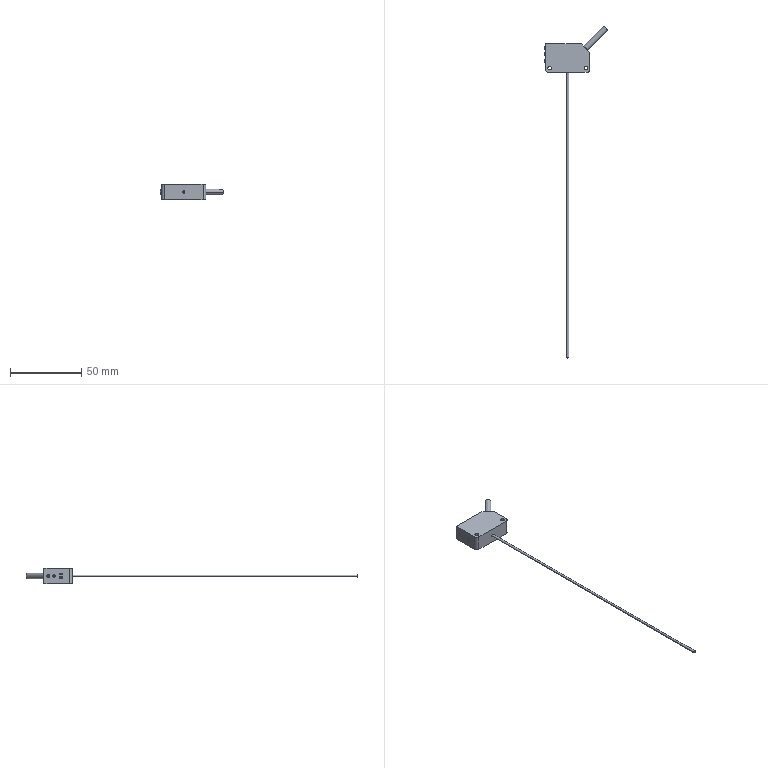Part | SolidWorks | features BaseBody 1 | 1 solid | 39 faces | box 44.556 x 232.556 x 10.8 mm | volume 6994 mm3 | cylinder 18 | plane 14 | spline 7 | commonest cylinder face diameters 2 x6 2.5 x4 4 x4 1 x2 1.5 x2
STEP:
#1=CARTESIAN_POINT('',(-0.6496,0.3346,0.03937));
#2=VERTEX_POINT('',#1);
#3=CARTESIAN_POINT('',(-0.6496,0.315,0.05906));
#4=VERTEX_POINT('',#3);
#5=CARTESIAN_POINT('',(-0.6496,0.3346,0.03937));
#6=CARTESIAN_POINT('',(-0.6496,0.3346,0.0509));
#7=CARTESIAN_POINT('',(-0.6496,0.3265,0.05906));
#8=CARTESIAN_POINT('',(-0.6496,0.315,0.05906));
#9=(BOUNDED_CURVE()B_SPLINE_CURVE(3,(#5,#6,#7,#8),.UNSPECIFIED.,.F.,.T.)B_SPLINE_CURVE_WITH_KNOTS((4,4),(0.,1.),.UNSPECIFIED.)CURVE()GEOMETRIC_REPRESENTATION_ITEM()RATIONAL_B_SPLINE_CURVE((1.,0.8047,0.8047,1.))REPRESENTATION_ITEM(''));
#10=EDGE_CURVE('',#2,#4,#9,.T.);
#11=ORIENTED_EDGE('',*,*,#10,.T.);
#12=CARTESIAN_POINT('',(-0.6299,0.315,0.07874));
#13=VERTEX_POINT('',#12);
#14=CARTESIAN_POINT('',(-0.6299,0.315,0.05906));
#15=DIRECTION('',(0.,1.,0.));
#16=DIRECTION('',(0.,0.,1.));
#17=AXIS2_PLACEMENT_3D('',#14,#15,#16);
#18=CIRCLE('',#17,0.01969);
#19=EDGE_CURVE('',#4,#13,#18,.T.);
#20=ORIENTED_EDGE('',*,*,#19,.T.);
#21=CARTESIAN_POINT('',(-0.6299,0.3543,0.03937));
#22=VERTEX_POINT('',#21);
#23=CARTESIAN_POINT('',(-0.6299,0.315,0.03937));
#24=DIRECTION('',(1.,0.,0.));
#25=DIRECTION('',(0.,1.,0.));
#26=AXIS2_PLACEMENT_3D('',#23,#24,#25);
#27=CIRCLE('',#26,0.03937);
#28=EDGE_CURVE('',#22,#13,#27,.T.);
#29=ORIENTED_EDGE('',*,*,#28,.F.);
#30=CARTESIAN_POINT('',(-0.6299,0.3346,0.03937));
#31=DIRECTION('',(0.,0.,-1.));
#32=DIRECTION('',(0.,-1.,0.));
#33=AXIS2_PLACEMENT_3D('',#30,#31,#32);
#34=CIRCLE('',#33,0.01969);
#35=EDGE_CURVE('',#2,#22,#34,.T.);
#36=ORIENTED_EDGE('',*,*,#35,.F.);
#37=EDGE_LOOP('',(#11,#20,#29,#36));
#38=FACE_OUTER_BOUND('',#37,.T.);
#39=CARTESIAN_POINT('',(-0.6496,0.315,0.05906));
#40=CARTESIAN_POINT('',(-0.6496,0.3265,0.05906));
#41=CARTESIAN_POINT('',(-0.6496,0.3346,0.0509));
#42=CARTESIAN_POINT('',(-0.6496,0.3346,0.03937));
#43=CARTESIAN_POINT('',(-0.6496,0.315,0.07059));
#44=CARTESIAN_POINT('',(-0.6496,0.3332,0.07059));
#45=CARTESIAN_POINT('',(-0.6496,0.3462,0.05766));
#46=CARTESIAN_POINT('',(-0.6496,0.3462,0.03937));
#47=CARTESIAN_POINT('',(-0.6415,0.315,0.07874));
#48=CARTESIAN_POINT('',(-0.6415,0.338,0.07874));
#49=CARTESIAN_POINT('',(-0.6415,0.3543,0.06243));
#50=CARTESIAN_POINT('',(-0.6415,0.3543,0.03937));
#51=CARTESIAN_POINT('',(-0.6299,0.315,0.07874));
#52=CARTESIAN_POINT('',(-0.6299,0.338,0.07874));
#53=CARTESIAN_POINT('',(-0.6299,0.3543,0.06243));
#54=CARTESIAN_POINT('',(-0.6299,0.3543,0.03937));
#55=(BOUNDED_SURFACE()B_SPLINE_SURFACE(3,3,((#39,#40,#41,#42),(#43,#44,#45,#46),(#47,#48,#49,#50),(#51,#52,#53,#54)),.UNSPECIFIED.,.F.,.F.,.F.)B_SPLINE_SURFACE_WITH_KNOTS((4,4),(4,4),(0.,1.),(0.,1.),.UNSPECIFIED.)GEOMETRIC_REPRESENTATION_ITEM()RATIONAL_B_SPLINE_SURFACE(((1.,0.8047,0.8047,1.),(0.8047,0.6476,0.6476,0.8047),(0.8047,0.6476,0.6476,0.8047),(1.,0.8047,0.8047,1.)))REPRESENTATION_ITEM('')SURFACE());
#56=ADVANCED_FACE('',(#38),#55,.T.);
#57=CARTESIAN_POINT('',(-0.6496,0.5118,0.01969));
#58=VERTEX_POINT('',#57);
#59=CARTESIAN_POINT('',(-0.6496,0.5118,-0.01969));
#60=VERTEX_POINT('',#59);
#61=CARTESIAN_POINT('',(-0.6496,0.5118,0.01969));
#62=CARTESIAN_POINT('',(-0.6496,0.4724,0.01969));
#63=CARTESIAN_POINT('',(-0.6496,0.4724,-0.01969));
#64=CARTESIAN_POINT('',(-0.6496,0.5118,-0.01969));
#65=(BOUNDED_CURVE()B_SPLINE_CURVE(3,(#61,#62,#63,#64),.UNSPECIFIED.,.F.,.F.)B_SPLINE_CURVE_WITH_KNOTS((4,4),(0.,1.),.UNSPECIFIED.)CURVE()GEOMETRIC_REPRESENTATION_ITEM()RATIONAL_B_SPLINE_CURVE((1.,0.3333,0.3333,1.))REPRESENTATION_ITEM(''));
#66=EDGE_CURVE('',#58,#60,#65,.T.);
#67=ORIENTED_EDGE('',*,*,#66,.T.);
#68=CARTESIAN_POINT('',(-0.6299,0.5118,-0.03937));
#69=VERTEX_POINT('',#68);
#70=CARTESIAN_POINT('',(-0.6299,0.5118,-0.01969));
#71=DIRECTION('',(0.,-1.,0.));
#72=DIRECTION('',(0.,0.,-1.));
#73=AXIS2_PLACEMENT_3D('',#70,#71,#72);
#74=CIRCLE('',#73,0.01969);
#75=EDGE_CURVE('',#60,#69,#74,.T.);
#76=ORIENTED_EDGE('',*,*,#75,.T.);
#77=CARTESIAN_POINT('',(-0.6299,0.4724,0.));
#78=VERTEX_POINT('',#77);
#79=CARTESIAN_POINT('',(-0.6299,0.5118,0.));
#80=DIRECTION('',(1.,0.,0.));
#81=DIRECTION('',(0.,1.,0.));
#82=AXIS2_PLACEMENT_3D('',#79,#80,#81);
#83=CIRCLE('',#82,0.03937);
#84=EDGE_CURVE('',#78,#69,#83,.T.);
#85=ORIENTED_EDGE('',*,*,#84,.F.);
#86=CARTESIAN_POINT('',(-0.6299,0.5118,0.03937));
#87=VERTEX_POINT('',#86);
#88=CARTESIAN_POINT('',(-0.6299,0.5118,0.));
#89=DIRECTION('',(1.,0.,0.));
#90=DIRECTION('',(0.,1.,0.));
#91=AXIS2_PLACEMENT_3D('',#88,#89,#90);
#92=CIRCLE('',#91,0.03937);
#93=EDGE_CURVE('',#87,#78,#92,.T.);
#94=ORIENTED_EDGE('',*,*,#93,.F.);
#95=CARTESIAN_POINT('',(-0.6299,0.5118,0.01969));
#96=DIRECTION('',(0.,1.,0.));
#97=DIRECTION('',(0.,0.,1.));
#98=AXIS2_PLACEMENT_3D('',#95,#96,#97);
#99=CIRCLE('',#98,0.01969);
#100=EDGE_CURVE('',#58,#87,#99,.T.);
#101=ORIENTED_EDGE('',*,*,#100,.F.);
#102=EDGE_LOOP('',(#67,#76,#85,#94,#101));
#103=FACE_OUTER_BOUND('',#102,.T.);
#104=CARTESIAN_POINT('',(-0.6496,0.5118,-0.01969));
#105=CARTESIAN_POINT('',(-0.6496,0.4724,-0.01969));
#106=CARTESIAN_POINT('',(-0.6496,0.4724,0.01969));
#107=CARTESIAN_POINT('',(-0.6496,0.5118,0.01969));
#108=CARTESIAN_POINT('',(-0.6496,0.5118,-0.03122));
#109=CARTESIAN_POINT('',(-0.6496,0.4494,-0.03122));
#110=CARTESIAN_POINT('',(-0.6496,0.4494,0.03122));
#111=CARTESIAN_POINT('',(-0.6496,0.5118,0.03122));
#112=CARTESIAN_POINT('',(-0.6415,0.5118,-0.03937));
#113=CARTESIAN_POINT('',(-0.6415,0.4331,-0.03937));
#114=CARTESIAN_POINT('',(-0.6415,0.4331,0.03937));
#115=CARTESIAN_POINT('',(-0.6415,0.5118,0.03937));
#116=CARTESIAN_POINT('',(-0.6299,0.5118,-0.03937));
#117=CARTESIAN_POINT('',(-0.6299,0.4331,-0.03937));
#118=CARTESIAN_POINT('',(-0.6299,0.4331,0.03937));
#119=CARTESIAN_POINT('',(-0.6299,0.5118,0.03937));
#120=(BOUNDED_SURFACE()B_SPLINE_SURFACE(3,3,((#104,#105,#106,#107),(#108,#109,#110,#111),(#112,#113,#114,#115),(#116,#117,#118,#119)),.UNSPECIFIED.,.F.,.F.,.F.)B_SPLINE_SURFACE_WITH_KNOTS((4,4),(4,4),(0.,1.),(0.,1.),.UNSPECIFIED.)GEOMETRIC_REPRESENTATION_ITEM()RATIONAL_B_SPLINE_SURFACE(((1.,0.3333,0.3333,1.),(0.8047,0.2682,0.2682,0.8047),(0.8047,0.2682,0.2682,0.8047),(1.,0.3333,0.3333,1.)))REPRESENTATION_ITEM('')SURFACE());
#121=ADVANCED_FACE('',(#103),#120,.T.);
#122=CARTESIAN_POINT('',(-0.6496,0.6693,0.01969));
#123=VERTEX_POINT('',#122);
#124=CARTESIAN_POINT('',(-0.6496,0.6693,-0.01969));
#125=VERTEX_POINT('',#124);
#126=CARTESIAN_POINT('',(-0.6496,0.6693,0.01969));
#127=CARTESIAN_POINT('',(-0.6496,0.6299,0.01969));
#128=CARTESIAN_POINT('',(-0.6496,0.6299,-0.01969));
#129=CARTESIAN_POINT('',(-0.6496,0.6693,-0.01969));
#130=(BOUNDED_CURVE()B_SPLINE_CURVE(3,(#126,#127,#128,#129),.UNSPECIFIED.,.F.,.T.)B_SPLINE_CURVE_WITH_KNOTS((4,4),(0.,1.),.UNSPECIFIED.)CURVE()GEOMETRIC_REPRESENTATION_ITEM()RATIONAL_B_SPLINE_CURVE((1.,0.3333,0.3333,1.))REPRESENTATION_ITEM(''));
#131=EDGE_CURVE('',#123,#125,#130,.T.);
#132=ORIENTED_EDGE('',*,*,#131,.T.);
#133=CARTESIAN_POINT('',(-0.6299,0.6693,-0.03937));
#134=VERTEX_POINT('',#133);
#135=CARTESIAN_POINT('',(-0.6299,0.6693,-0.01969));
#136=DIRECTION('',(0.,-1.,0.));
#137=DIRECTION('',(0.,0.,-1.));
#138=AXIS2_PLACEMENT_3D('',#135,#136,#137);
#139=CIRCLE('',#138,0.01969);
#140=EDGE_CURVE('',#125,#134,#139,.T.);
#141=ORIENTED_EDGE('',*,*,#140,.T.);
#142=CARTESIAN_POINT('',(-0.6299,0.6299,0.));
#143=VERTEX_POINT('',#142);
#144=CARTESIAN_POINT('',(-0.6299,0.6693,0.));
#145=DIRECTION('',(1.,0.,0.));
#146=DIRECTION('',(0.,1.,0.));
#147=AXIS2_PLACEMENT_3D('',#144,#145,#146);
#148=CIRCLE('',#147,0.03937);
#149=EDGE_CURVE('',#143,#134,#148,.T.);
#150=ORIENTED_EDGE('',*,*,#149,.F.);
#151=CARTESIAN_POINT('',(-0.6299,0.6693,0.03937));
#152=VERTEX_POINT('',#151);
#153=CARTESIAN_POINT('',(-0.6299,0.6693,0.));
#154=DIRECTION('',(1.,0.,0.));
#155=DIRECTION('',(0.,1.,0.));
#156=AXIS2_PLACEMENT_3D('',#153,#154,#155);
#157=CIRCLE('',#156,0.03937);
#158=EDGE_CURVE('',#152,#143,#157,.T.);
#159=ORIENTED_EDGE('',*,*,#158,.F.);
#160=CARTESIAN_POINT('',(-0.6299,0.6693,0.01969));
#161=DIRECTION('',(0.,1.,0.));
#162=DIRECTION('',(0.,0.,1.));
#163=AXIS2_PLACEMENT_3D('',#160,#161,#162);
#164=CIRCLE('',#163,0.01969);
#165=EDGE_CURVE('',#123,#152,#164,.T.);
#166=ORIENTED_EDGE('',*,*,#165,.F.);
#167=EDGE_LOOP('',(#132,#141,#150,#159,#166));
#168=FACE_OUTER_BOUND('',#167,.T.);
#169=CARTESIAN_POINT('',(-0.6496,0.6693,-0.01969));
#170=CARTESIAN_POINT('',(-0.6496,0.6299,-0.01969));
#171=CARTESIAN_POINT('',(-0.6496,0.6299,0.01969));
#172=CARTESIAN_POINT('',(-0.6496,0.6693,0.01969));
#173=CARTESIAN_POINT('',(-0.6496,0.6693,-0.03122));
#174=CARTESIAN_POINT('',(-0.6496,0.6069,-0.03122));
#175=CARTESIAN_POINT('',(-0.6496,0.6069,0.03122));
#176=CARTESIAN_POINT('',(-0.6496,0.6693,0.03122));
#177=CARTESIAN_POINT('',(-0.6415,0.6693,-0.03937));
#178=CARTESIAN_POINT('',(-0.6415,0.5906,-0.03937));
#179=CARTESIAN_POINT('',(-0.6415,0.5906,0.03937));
#180=CARTESIAN_POINT('',(-0.6415,0.6693,0.03937));
#181=CARTESIAN_POINT('',(-0.6299,0.6693,-0.03937));
#182=CARTESIAN_POINT('',(-0.6299,0.5906,-0.03937));
#183=CARTESIAN_POINT('',(-0.6299,0.5906,0.03937));
#184=CARTESIAN_POINT('',(-0.6299,0.6693,0.03937));
#185=(BOUNDED_SURFACE()B_SPLINE_SURFACE(3,3,((#169,#170,#171,#172),(#173,#174,#175,#176),(#177,#178,#179,#180),(#181,#182,#183,#184)),.UNSPECIFIED.,.F.,.F.,.F.)B_SPLINE_SURFACE_WITH_KNOTS((4,4),(4,4),(0.,1.),(0.,1.),.UNSPECIFIED.)GEOMETRIC_REPRESENTATION_ITEM()RATIONAL_B_SPLINE_SURFACE(((1.,0.3333,0.3333,1.),(0.8047,0.2682,0.2682,0.8047),(0.8047,0.2682,0.2682,0.8047),(1.,0.3333,0.3333,1.)))REPRESENTATION_ITEM('')SURFACE());
#186=ADVANCED_FACE('',(#168),#185,.T.);
#187=CARTESIAN_POINT('',(0.5,0.1673,-0.2126));
#188=VERTEX_POINT('',#187);
#189=CARTESIAN_POINT('',(0.5,0.0689,-0.2126));
#190=VERTEX_POINT('',#189);
#191=CARTESIAN_POINT('',(0.5,0.1181,-0.2126));
#192=DIRECTION('',(0.,0.,1.));
#193=DIRECTION('',(0.,-1.,0.));
#194=AXIS2_PLACEMENT_3D('',#191,#192,#193);
#195=CIRCLE('',#194,0.04921);
#196=EDGE_CURVE('',#188,#190,#195,.T.);
#197=ORIENTED_EDGE('',*,*,#196,.F.);
#198=CARTESIAN_POINT('',(0.5,0.1673,0.2126));
#199=VERTEX_POINT('',#198);
#200=CARTESIAN_POINT('',(0.5,0.1673,0.2126));
#201=DIRECTION('',(0.,0.,1.));
#202=VECTOR('',#201,39.37);
#203=LINE('',#200,#202);
#204=EDGE_CURVE('',#188,#199,#203,.T.);
#205=ORIENTED_EDGE('',*,*,#204,.T.);
#206=CARTESIAN_POINT('',(0.5,0.0689,0.2126));
#207=VERTEX_POINT('',#206);
#208=CARTESIAN_POINT('',(0.5,0.1181,0.2126));
#209=DIRECTION('',(0.,0.,-1.));
#210=DIRECTION('',(0.,-1.,0.));
#211=AXIS2_PLACEMENT_3D('',#208,#209,#210);
#212=CIRCLE('',#211,0.04921);
#213=EDGE_CURVE('',#207,#199,#212,.T.);
#214=ORIENTED_EDGE('',*,*,#213,.F.);
#215=CARTESIAN_POINT('',(0.5,0.0689,0.2126));
#216=DIRECTION('',(0.,0.,1.));
#217=VECTOR('',#216,39.37);
#218=LINE('',#215,#217);
#219=EDGE_CURVE('',#190,#207,#218,.T.);
#220=ORIENTED_EDGE('',*,*,#219,.F.);
#221=EDGE_LOOP('',(#197,#205,#214,#220));
#222=FACE_OUTER_BOUND('',#221,.T.);
#223=CARTESIAN_POINT('',(0.5,0.1181,0.2126));
#224=DIRECTION('',(0.,0.,1.));
#225=DIRECTION('',(0.,-1.,0.));
#226=AXIS2_PLACEMENT_3D('',#223,#224,#225);
#227=CYLINDRICAL_SURFACE('',#226,0.04921);
#228=ADVANCED_FACE('',(#222),#227,.F.);
#229=CARTESIAN_POINT('',(-0.5,0.1673,-0.2126));
#230=VERTEX_POINT('',#229);
#231=CARTESIAN_POINT('',(-0.5,0.0689,-0.2126));
#232=VERTEX_POINT('',#231);
#233=CARTESIAN_POINT('',(-0.5,0.1181,-0.2126));
#234=DIRECTION('',(0.,0.,1.));
#235=DIRECTION('',(0.,-1.,0.));
#236=AXIS2_PLACEMENT_3D('',#233,#234,#235);
#237=CIRCLE('',#236,0.04921);
#238=EDGE_CURVE('',#230,#232,#237,.T.);
#239=ORIENTED_EDGE('',*,*,#238,.F.);
#240=CARTESIAN_POINT('',(-0.5,0.1673,0.2126));
#241=VERTEX_POINT('',#240);
#242=CARTESIAN_POINT('',(-0.5,0.1673,0.2126));
#243=DIRECTION('',(0.,0.,1.));
#244=VECTOR('',#243,39.37);
#245=LINE('',#242,#244);
#246=EDGE_CURVE('',#230,#241,#245,.T.);
#247=ORIENTED_EDGE('',*,*,#246,.T.);
#248=CARTESIAN_POINT('',(-0.5,0.0689,0.2126));
#249=VERTEX_POINT('',#248);
#250=CARTESIAN_POINT('',(-0.5,0.1181,0.2126));
#251=DIRECTION('',(0.,0.,-1.));
#252=DIRECTION('',(0.,-1.,0.));
#253=AXIS2_PLACEMENT_3D('',#250,#251,#252);
#254=CIRCLE('',#253,0.04921);
#255=EDGE_CURVE('',#249,#241,#254,.T.);
#256=ORIENTED_EDGE('',*,*,#255,.F.);
#257=CARTESIAN_POINT('',(-0.5,0.0689,0.2126));
#258=DIRECTION('',(0.,0.,1.));
#259=VECTOR('',#258,39.37);
#260=LINE('',#257,#259);
#261=EDGE_CURVE('',#232,#249,#260,.T.);
#262=ORIENTED_EDGE('',*,*,#261,.F.);
#263=EDGE_LOOP('',(#239,#247,#256,#262));
#264=FACE_OUTER_BOUND('',#263,.T.);
#265=CARTESIAN_POINT('',(-0.5,0.1181,0.2126));
#266=DIRECTION('',(0.,0.,1.));
#267=DIRECTION('',(0.,-1.,0.));
#268=AXIS2_PLACEMENT_3D('',#265,#266,#267);
#269=CYLINDRICAL_SURFACE('',#268,0.04921);
#270=ADVANCED_FACE('',(#264),#269,.F.);
#271=CARTESIAN_POINT('',(1.105,1.17,0.));
#272=VERTEX_POINT('',#271);
#273=CARTESIAN_POINT('',(0.9932,1.282,0.));
#274=VERTEX_POINT('',#273);
#275=CARTESIAN_POINT('',(1.049,1.226,0.));
#276=DIRECTION('',(-0.7071,-0.7071,0.));
#277=DIRECTION('',(0.7071,-0.7071,0.));
#278=AXIS2_PLACEMENT_3D('',#275,#276,#277);
#279=CIRCLE('',#278,0.07874);
#280=EDGE_CURVE('',#272,#274,#279,.T.);
#281=ORIENTED_EDGE('',*,*,#280,.T.);
#282=CARTESIAN_POINT('',(0.4364,0.725,0.));
#283=VERTEX_POINT('',#282);
#284=CARTESIAN_POINT('',(0.9932,1.282,0.));
#285=DIRECTION('',(-0.7071,-0.7071,0.));
#286=VECTOR('',#285,39.37);
#287=LINE('',#284,#286);
#288=EDGE_CURVE('',#274,#283,#287,.T.);
#289=ORIENTED_EDGE('',*,*,#288,.T.);
#290=CARTESIAN_POINT('',(0.5478,0.6136,0.));
#291=VERTEX_POINT('',#290);
#292=CARTESIAN_POINT('',(0.4921,0.6693,0.));
#293=DIRECTION('',(0.7071,0.7071,0.));
#294=DIRECTION('',(0.7071,-0.7071,0.));
#295=AXIS2_PLACEMENT_3D('',#292,#293,#294);
#296=CIRCLE('',#295,0.07874);
#297=EDGE_CURVE('',#283,#291,#296,.T.);
#298=ORIENTED_EDGE('',*,*,#297,.T.);
#299=CARTESIAN_POINT('',(1.105,1.17,0.));
#300=DIRECTION('',(-0.7071,-0.7071,0.));
#301=VECTOR('',#300,39.37);
#302=LINE('',#299,#301);
#303=EDGE_CURVE('',#272,#291,#302,.T.);
#304=ORIENTED_EDGE('',*,*,#303,.F.);
#305=EDGE_LOOP('',(#281,#289,#298,#304));
#306=FACE_OUTER_BOUND('',#305,.T.);
#307=CARTESIAN_POINT('',(1.049,1.226,0.));
#308=DIRECTION('',(-0.7071,-0.7071,0.));
#309=DIRECTION('',(0.7071,-0.7071,0.));
#310=AXIS2_PLACEMENT_3D('',#307,#308,#309);
#311=CYLINDRICAL_SURFACE('',#310,0.07874);
#312=ADVANCED_FACE('',(#306),#311,.T.);
#313=CARTESIAN_POINT('',(-0.6299,0.5512,0.));
#314=VERTEX_POINT('',#313);
#315=CARTESIAN_POINT('',(-0.6299,0.5118,0.));
#316=DIRECTION('',(1.,0.,0.));
#317=DIRECTION('',(0.,1.,0.));
#318=AXIS2_PLACEMENT_3D('',#315,#316,#317);
#319=CIRCLE('',#318,0.03937);
#320=EDGE_CURVE('',#314,#87,#319,.T.);
#321=ORIENTED_EDGE('',*,*,#320,.T.);
#322=ORIENTED_EDGE('',*,*,#93,.T.);
#323=CARTESIAN_POINT('',(-0.6102,0.4724,0.));
#324=VERTEX_POINT('',#323);
#325=CARTESIAN_POINT('',(-0.6496,0.4724,0.));
#326=DIRECTION('',(1.,0.,0.));
#327=VECTOR('',#326,39.37);
#328=LINE('',#325,#327);
#329=EDGE_CURVE('',#78,#324,#328,.T.);
#330=ORIENTED_EDGE('',*,*,#329,.T.);
#331=CARTESIAN_POINT('',(-0.6102,0.5512,0.));
#332=VERTEX_POINT('',#331);
#333=CARTESIAN_POINT('',(-0.6102,0.5118,0.));
#334=DIRECTION('',(-1.,0.,0.));
#335=DIRECTION('',(0.,1.,0.));
#336=AXIS2_PLACEMENT_3D('',#333,#334,#335);
#337=CIRCLE('',#336,0.03937);
#338=EDGE_CURVE('',#324,#332,#337,.T.);
#339=ORIENTED_EDGE('',*,*,#338,.T.);
#340=CARTESIAN_POINT('',(-0.6496,0.5512,0.));
#341=DIRECTION('',(1.,0.,0.));
#342=VECTOR('',#341,39.37);
#343=LINE('',#340,#342);
#344=EDGE_CURVE('',#314,#332,#343,.T.);
#345=ORIENTED_EDGE('',*,*,#344,.F.);
#346=EDGE_LOOP('',(#321,#322,#330,#339,#345));
#347=FACE_OUTER_BOUND('',#346,.T.);
#348=CARTESIAN_POINT('',(-0.6496,0.5118,0.));
#349=DIRECTION('',(1.,0.,0.));
#350=DIRECTION('',(0.,1.,0.));
#351=AXIS2_PLACEMENT_3D('',#348,#349,#350);
#352=CYLINDRICAL_SURFACE('',#351,0.03937);
#353=ADVANCED_FACE('',(#347),#352,.T.);
#354=CARTESIAN_POINT('',(-0.6299,0.7087,0.));
#355=VERTEX_POINT('',#354);
#356=CARTESIAN_POINT('',(-0.6299,0.6693,0.));
#357=DIRECTION('',(1.,0.,0.));
#358=DIRECTION('',(0.,1.,0.));
#359=AXIS2_PLACEMENT_3D('',#356,#357,#358);
#360=CIRCLE('',#359,0.03937);
#361=EDGE_CURVE('',#355,#152,#360,.T.);
#362=ORIENTED_EDGE('',*,*,#361,.T.);
#363=ORIENTED_EDGE('',*,*,#158,.T.);
#364=CARTESIAN_POINT('',(-0.6102,0.6299,0.));
#365=VERTEX_POINT('',#364);
#366=CARTESIAN_POINT('',(-0.6496,0.6299,0.));
#367=DIRECTION('',(1.,0.,0.));
#368=VECTOR('',#367,39.37);
#369=LINE('',#366,#368);
#370=EDGE_CURVE('',#143,#365,#369,.T.);
#371=ORIENTED_EDGE('',*,*,#370,.T.);
#372=CARTESIAN_POINT('',(-0.6102,0.7087,0.));
#373=VERTEX_POINT('',#372);
#374=CARTESIAN_POINT('',(-0.6102,0.6693,0.));
#375=DIRECTION('',(-1.,0.,0.));
#376=DIRECTION('',(0.,1.,0.));
#377=AXIS2_PLACEMENT_3D('',#374,#375,#376);
#378=CIRCLE('',#377,0.03937);
#379=EDGE_CURVE('',#365,#373,#378,.T.);
#380=ORIENTED_EDGE('',*,*,#379,.T.);
#381=CARTESIAN_POINT('',(-0.6496,0.7087,0.));
#382=DIRECTION('',(1.,0.,0.));
#383=VECTOR('',#382,39.37);
#384=LINE('',#381,#383);
#385=EDGE_CURVE('',#355,#373,#384,.T.);
#386=ORIENTED_EDGE('',*,*,#385,.F.);
#387=EDGE_LOOP('',(#362,#363,#371,#380,#386));
#388=FACE_OUTER_BOUND('',#387,.T.);
#389=CARTESIAN_POINT('',(-0.6496,0.6693,0.));
#390=DIRECTION('',(1.,0.,0.));
#391=DIRECTION('',(0.,1.,0.));
#392=AXIS2_PLACEMENT_3D('',#389,#390,#391);
#393=CYLINDRICAL_SURFACE('',#392,0.03937);
#394=ADVANCED_FACE('',(#388),#393,.T.);
#395=CARTESIAN_POINT('',(-0.02953,-7.874,0.));
#396=VERTEX_POINT('',#395);
#397=CARTESIAN_POINT('',(0.02953,-7.874,0.));
#398=VERTEX_POINT('',#397);
#399=CARTESIAN_POINT('',(0.,-7.874,0.));
#400=DIRECTION('',(0.,1.,0.));
#401=DIRECTION('',(-1.,0.,0.));
#402=AXIS2_PLACEMENT_3D('',#399,#400,#401);
#403=CIRCLE('',#402,0.02953);
#404=EDGE_CURVE('',#396,#398,#403,.T.);
#405=ORIENTED_EDGE('',*,*,#404,.T.);
#406=CARTESIAN_POINT('',(0.02953,0.,0.));
#407=VERTEX_POINT('',#406);
#408=CARTESIAN_POINT('',(0.02953,-7.874,0.));
#409=DIRECTION('',(0.,1.,0.));
#410=VECTOR('',#409,39.37);
#411=LINE('',#408,#410);
#412=EDGE_CURVE('',#398,#407,#411,.T.);
#413=ORIENTED_EDGE('',*,*,#412,.T.);
#414=CARTESIAN_POINT('',(-0.02953,0.,0.));
#415=VERTEX_POINT('',#414);
#416=CARTESIAN_POINT('',(0.,0.,0.));
#417=DIRECTION('',(0.,-1.,0.));
#418=DIRECTION('',(-1.,0.,0.));
#419=AXIS2_PLACEMENT_3D('',#416,#417,#418);
#420=CIRCLE('',#419,0.02953);
#421=EDGE_CURVE('',#407,#415,#420,.T.);
#422=ORIENTED_EDGE('',*,*,#421,.T.);
#423=CARTESIAN_POINT('',(-0.02953,-7.874,0.));
#424=DIRECTION('',(0.,1.,0.));
#425=VECTOR('',#424,39.37);
#426=LINE('',#423,#425);
#427=EDGE_CURVE('',#396,#415,#426,.T.);
#428=ORIENTED_EDGE('',*,*,#427,.F.);
#429=EDGE_LOOP('',(#405,#413,#422,#428));
#430=FACE_OUTER_BOUND('',#429,.T.);
#431=CARTESIAN_POINT('',(0.,-7.874,0.));
#432=DIRECTION('',(0.,1.,0.));
#433=DIRECTION('',(-1.,0.,0.));
#434=AXIS2_PLACEMENT_3D('',#431,#432,#433);
#435=CYLINDRICAL_SURFACE('',#434,0.02953);
#436=ADVANCED_FACE('',(#430),#435,.T.);
#437=CARTESIAN_POINT('',(0.6102,0.5512,-0.2126));
#438=VERTEX_POINT('',#437);
#439=CARTESIAN_POINT('',(0.6102,0.07874,-0.2126));
#440=VERTEX_POINT('',#439);
#441=CARTESIAN_POINT('',(0.6102,0.,-0.2126));
#442=DIRECTION('',(0.,-1.,0.));
#443=VECTOR('',#442,39.37);
#444=LINE('',#441,#443);
#445=EDGE_CURVE('',#438,#440,#444,.T.);
#446=ORIENTED_EDGE('',*,*,#445,.T.);
#447=CARTESIAN_POINT('',(0.5315,0.,-0.2126));
#448=VERTEX_POINT('',#447);
#449=CARTESIAN_POINT('',(0.5315,0.07874,-0.2126));
#450=DIRECTION('',(0.,0.,-1.));
#451=DIRECTION('',(0.,1.,0.));
#452=AXIS2_PLACEMENT_3D('',#449,#450,#451);
#453=CIRCLE('',#452,0.07874);
#454=EDGE_CURVE('',#440,#448,#453,.T.);
#455=ORIENTED_EDGE('',*,*,#454,.T.);
#456=CARTESIAN_POINT('',(-0.5315,0.,-0.2126));
#457=VERTEX_POINT('',#456);
#458=CARTESIAN_POINT('',(0.,0.,-0.2126));
#459=DIRECTION('',(-1.,0.,0.));
#460=VECTOR('',#459,39.37);
#461=LINE('',#458,#460);
#462=EDGE_CURVE('',#448,#457,#461,.T.);
#463=ORIENTED_EDGE('',*,*,#462,.T.);
#464=CARTESIAN_POINT('',(-0.6102,0.07874,-0.2126));
#465=VERTEX_POINT('',#464);
#466=CARTESIAN_POINT('',(-0.5315,0.07874,-0.2126));
#467=DIRECTION('',(0.,0.,-1.));
#468=DIRECTION('',(0.,1.,0.));
#469=AXIS2_PLACEMENT_3D('',#466,#467,#468);
#470=CIRCLE('',#469,0.07874);
#471=EDGE_CURVE('',#457,#465,#470,.T.);
#472=ORIENTED_EDGE('',*,*,#471,.T.);
#473=CARTESIAN_POINT('',(-0.6102,0.7874,-0.2126));
#474=VERTEX_POINT('',#473);
#475=CARTESIAN_POINT('',(-0.6102,0.,-0.2126));
#476=DIRECTION('',(0.,1.,0.));
#477=VECTOR('',#476,39.37);
#478=LINE('',#475,#477);
#479=EDGE_CURVE('',#465,#474,#478,.T.);
#480=ORIENTED_EDGE('',*,*,#479,.T.);
#481=CARTESIAN_POINT('',(0.374,0.7874,-0.2126));
#482=VERTEX_POINT('',#481);
#483=CARTESIAN_POINT('',(0.,0.7874,-0.2126));
#484=DIRECTION('',(1.,0.,0.));
#485=VECTOR('',#484,39.37);
#486=LINE('',#483,#485);
#487=EDGE_CURVE('',#474,#482,#486,.T.);
#488=ORIENTED_EDGE('',*,*,#487,.T.);
#489=CARTESIAN_POINT('',(0.374,0.7874,-0.2126));
#490=DIRECTION('',(0.7071,-0.7071,0.));
#491=VECTOR('',#490,39.37);
#492=LINE('',#489,#491);
#493=EDGE_CURVE('',#482,#438,#492,.T.);
#494=ORIENTED_EDGE('',*,*,#493,.T.);
#495=EDGE_LOOP('',(#446,#455,#463,#472,#480,#488,#494));
#496=FACE_OUTER_BOUND('',#495,.T.);
#497=CARTESIAN_POINT('',(0.5,0.1181,-0.2126));
#498=DIRECTION('',(0.,0.,1.));
#499=DIRECTION('',(0.,-1.,0.));
#500=AXIS2_PLACEMENT_3D('',#497,#498,#499);
#501=CIRCLE('',#500,0.04921);
#502=EDGE_CURVE('',#190,#188,#501,.T.);
#503=ORIENTED_EDGE('',*,*,#502,.T.);
#504=ORIENTED_EDGE('',*,*,#196,.T.);
#505=EDGE_LOOP('',(#503,#504));
#506=FACE_BOUND('',#505,.T.);
#507=CARTESIAN_POINT('',(-0.5,0.1181,-0.2126));
#508=DIRECTION('',(0.,0.,1.));
#509=DIRECTION('',(0.,-1.,0.));
#510=AXIS2_PLACEMENT_3D('',#507,#508,#509);
#511=CIRCLE('',#510,0.04921);
#512=EDGE_CURVE('',#232,#230,#511,.T.);
#513=ORIENTED_EDGE('',*,*,#512,.T.);
#514=ORIENTED_EDGE('',*,*,#238,.T.);
#515=EDGE_LOOP('',(#513,#514));
#516=FACE_BOUND('',#515,.T.);
#517=CARTESIAN_POINT('',(0.,0.,-0.2126));
#518=DIRECTION('',(0.,0.,-1.));
#519=DIRECTION('',(0.,1.,0.));
#520=AXIS2_PLACEMENT_3D('',#517,#518,#519);
#521=PLANE('',#520);
#522=ADVANCED_FACE('',(#496,#506,#516),#521,.T.);
#523=ORIENTED_EDGE('',*,*,#454,.F.);
#524=CARTESIAN_POINT('',(0.6102,0.07874,0.2126));
#525=VERTEX_POINT('',#524);
#526=CARTESIAN_POINT('',(0.6102,0.07874,0.2126));
#527=DIRECTION('',(0.,0.,1.));
#528=VECTOR('',#527,39.37);
#529=LINE('',#526,#528);
#530=EDGE_CURVE('',#440,#525,#529,.T.);
#531=ORIENTED_EDGE('',*,*,#530,.T.);
#532=CARTESIAN_POINT('',(0.5315,0.,0.2126));
#533=VERTEX_POINT('',#532);
#534=CARTESIAN_POINT('',(0.5315,0.07874,0.2126));
#535=DIRECTION('',(0.,0.,-1.));
#536=DIRECTION('',(0.,1.,0.));
#537=AXIS2_PLACEMENT_3D('',#534,#535,#536);
#538=CIRCLE('',#537,0.07874);
#539=EDGE_CURVE('',#525,#533,#538,.T.);
#540=ORIENTED_EDGE('',*,*,#539,.T.);
#541=CARTESIAN_POINT('',(0.5315,0.,0.2126));
#542=DIRECTION('',(0.,0.,-1.));
#543=VECTOR('',#542,39.37);
#544=LINE('',#541,#543);
#545=EDGE_CURVE('',#533,#448,#544,.T.);
#546=ORIENTED_EDGE('',*,*,#545,.T.);
#547=EDGE_LOOP('',(#523,#531,#540,#546));
#548=FACE_OUTER_BOUND('',#547,.T.);
#549=CARTESIAN_POINT('',(0.5315,0.07874,0.2126));
#550=DIRECTION('',(0.,0.,-1.));
#551=DIRECTION('',(0.,1.,0.));
#552=AXIS2_PLACEMENT_3D('',#549,#550,#551);
#553=CYLINDRICAL_SURFACE('',#552,0.07874);
#554=ADVANCED_FACE('',(#548),#553,.T.);
#555=ORIENTED_EDGE('',*,*,#530,.F.);
#556=ORIENTED_EDGE('',*,*,#445,.F.);
#557=CARTESIAN_POINT('',(0.6102,0.5512,0.2126));
#558=VERTEX_POINT('',#557);
#559=CARTESIAN_POINT('',(0.6102,0.5512,0.2126));
#560=DIRECTION('',(0.,0.,-1.));
#561=VECTOR('',#560,39.37);
#562=LINE('',#559,#561);
#563=EDGE_CURVE('',#558,#438,#562,.T.);
#564=ORIENTED_EDGE('',*,*,#563,.F.);
#565=CARTESIAN_POINT('',(0.6102,0.,0.2126));
#566=DIRECTION('',(0.,1.,0.));
#567=VECTOR('',#566,39.37);
#568=LINE('',#565,#567);
#569=EDGE_CURVE('',#525,#558,#568,.T.);
#570=ORIENTED_EDGE('',*,*,#569,.F.);
#571=EDGE_LOOP('',(#555,#556,#564,#570));
#572=FACE_OUTER_BOUND('',#571,.T.);
#573=CARTESIAN_POINT('',(0.6102,0.,0.2126));
#574=DIRECTION('',(-1.,0.,0.));
#575=DIRECTION('',(0.,-1.,0.));
#576=AXIS2_PLACEMENT_3D('',#573,#574,#575);
#577=PLANE('',#576);
#578=ADVANCED_FACE('',(#572),#577,.F.);
#579=CARTESIAN_POINT('',(0.4921,0.6693,0.));
#580=DIRECTION('',(0.7071,0.7071,0.));
#581=DIRECTION('',(0.7071,-0.7071,0.));
#582=AXIS2_PLACEMENT_3D('',#579,#580,#581);
#583=CIRCLE('',#582,0.07874);
#584=EDGE_CURVE('',#291,#283,#583,.T.);
#585=ORIENTED_EDGE('',*,*,#584,.F.);
#586=ORIENTED_EDGE('',*,*,#297,.F.);
#587=EDGE_LOOP('',(#585,#586));
#588=FACE_BOUND('',#587,.T.);
#589=ORIENTED_EDGE('',*,*,#563,.T.);
#590=ORIENTED_EDGE('',*,*,#493,.F.);
#591=CARTESIAN_POINT('',(0.374,0.7874,0.2126));
#592=VERTEX_POINT('',#591);
#593=CARTESIAN_POINT('',(0.374,0.7874,0.2126));
#594=DIRECTION('',(0.,0.,-1.));
#595=VECTOR('',#594,39.37);
#596=LINE('',#593,#595);
#597=EDGE_CURVE('',#592,#482,#596,.T.);
#598=ORIENTED_EDGE('',*,*,#597,.F.);
#599=CARTESIAN_POINT('',(0.374,0.7874,0.2126));
#600=DIRECTION('',(-0.7071,0.7071,0.));
#601=VECTOR('',#600,39.37);
#602=LINE('',#599,#601);
#603=EDGE_CURVE('',#558,#592,#602,.T.);
#604=ORIENTED_EDGE('',*,*,#603,.F.);
#605=EDGE_LOOP('',(#589,#590,#598,#604));
#606=FACE_OUTER_BOUND('',#605,.T.);
#607=CARTESIAN_POINT('',(0.374,0.7874,0.2126));
#608=DIRECTION('',(-0.7071,-0.7071,0.));
#609=DIRECTION('',(0.7071,-0.7071,0.));
#610=AXIS2_PLACEMENT_3D('',#607,#608,#609);
#611=PLANE('',#610);
#612=ADVANCED_FACE('',(#588,#606),#611,.F.);
#613=ORIENTED_EDGE('',*,*,#597,.T.);
#614=ORIENTED_EDGE('',*,*,#487,.F.);
#615=CARTESIAN_POINT('',(-0.6102,0.7874,0.2126));
#616=VERTEX_POINT('',#615);
#617=CARTESIAN_POINT('',(-0.6102,0.7874,0.2126));
#618=DIRECTION('',(0.,0.,-1.));
#619=VECTOR('',#618,39.37);
#620=LINE('',#617,#619);
#621=EDGE_CURVE('',#616,#474,#620,.T.);
#622=ORIENTED_EDGE('',*,*,#621,.F.);
#623=CARTESIAN_POINT('',(-0.6102,0.7874,0.2126));
#624=DIRECTION('',(-1.,0.,0.));
#625=VECTOR('',#624,39.37);
#626=LINE('',#623,#625);
#627=EDGE_CURVE('',#592,#616,#626,.T.);
#628=ORIENTED_EDGE('',*,*,#627,.F.);
#629=EDGE_LOOP('',(#613,#614,#622,#628));
#630=FACE_OUTER_BOUND('',#629,.T.);
#631=CARTESIAN_POINT('',(-0.6102,0.7874,0.2126));
#632=DIRECTION('',(0.,-1.,0.));
#633=DIRECTION('',(1.,0.,0.));
#634=AXIS2_PLACEMENT_3D('',#631,#632,#633);
#635=PLANE('',#634);
#636=ADVANCED_FACE('',(#630),#635,.F.);
#637=CARTESIAN_POINT('',(-0.6102,0.3543,0.03937));
#638=VERTEX_POINT('',#637);
#639=CARTESIAN_POINT('',(-0.6102,0.3543,-0.03937));
#640=VERTEX_POINT('',#639);
#641=CARTESIAN_POINT('',(-0.6102,0.3543,0.2126));
#642=DIRECTION('',(0.,0.,-1.));
#643=VECTOR('',#642,39.37);
#644=LINE('',#641,#643);
#645=EDGE_CURVE('',#638,#640,#644,.T.);
#646=ORIENTED_EDGE('',*,*,#645,.F.);
#647=CARTESIAN_POINT('',(-0.6102,0.2756,0.03937));
#648=VERTEX_POINT('',#647);
#649=CARTESIAN_POINT('',(-0.6102,0.315,0.03937));
#650=DIRECTION('',(-1.,0.,0.));
#651=DIRECTION('',(0.,1.,0.));
#652=AXIS2_PLACEMENT_3D('',#649,#650,#651);
#653=CIRCLE('',#652,0.03937);
#654=EDGE_CURVE('',#648,#638,#653,.T.);
#655=ORIENTED_EDGE('',*,*,#654,.F.);
#656=CARTESIAN_POINT('',(-0.6102,0.2756,-0.03937));
#657=VERTEX_POINT('',#656);
#658=CARTESIAN_POINT('',(-0.6102,0.2756,0.2126));
#659=DIRECTION('',(0.,0.,1.));
#660=VECTOR('',#659,39.37);
#661=LINE('',#658,#660);
#662=EDGE_CURVE('',#657,#648,#661,.T.);
#663=ORIENTED_EDGE('',*,*,#662,.F.);
#664=CARTESIAN_POINT('',(-0.6102,0.315,-0.03937));
#665=DIRECTION('',(-1.,0.,0.));
#666=DIRECTION('',(0.,1.,0.));
#667=AXIS2_PLACEMENT_3D('',#664,#665,#666);
#668=CIRCLE('',#667,0.03937);
#669=EDGE_CURVE('',#640,#657,#668,.T.);
#670=ORIENTED_EDGE('',*,*,#669,.F.);
#671=EDGE_LOOP('',(#646,#655,#663,#670));
#672=FACE_BOUND('',#671,.T.);
#673=CARTESIAN_POINT('',(-0.6102,0.5118,0.));
#674=DIRECTION('',(-1.,0.,0.));
#675=DIRECTION('',(0.,1.,0.));
#676=AXIS2_PLACEMENT_3D('',#673,#674,#675);
#677=CIRCLE('',#676,0.03937);
#678=EDGE_CURVE('',#332,#324,#677,.T.);
#679=ORIENTED_EDGE('',*,*,#678,.F.);
#680=ORIENTED_EDGE('',*,*,#338,.F.);
#681=EDGE_LOOP('',(#679,#680));
#682=FACE_BOUND('',#681,.T.);
#683=CARTESIAN_POINT('',(-0.6102,0.07874,0.2126));
#684=VERTEX_POINT('',#683);
#685=CARTESIAN_POINT('',(-0.6102,0.07874,0.2126));
#686=DIRECTION('',(0.,0.,-1.));
#687=VECTOR('',#686,39.37);
#688=LINE('',#685,#687);
#689=EDGE_CURVE('',#684,#465,#688,.T.);
#690=ORIENTED_EDGE('',*,*,#689,.F.);
#691=CARTESIAN_POINT('',(-0.6102,0.,0.2126));
#692=DIRECTION('',(0.,-1.,0.));
#693=VECTOR('',#692,39.37);
#694=LINE('',#691,#693);
#695=EDGE_CURVE('',#616,#684,#694,.T.);
#696=ORIENTED_EDGE('',*,*,#695,.F.);
#697=ORIENTED_EDGE('',*,*,#621,.T.);
#698=ORIENTED_EDGE('',*,*,#479,.F.);
#699=EDGE_LOOP('',(#690,#696,#697,#698));
#700=FACE_OUTER_BOUND('',#699,.T.);
#701=CARTESIAN_POINT('',(-0.6102,0.6693,0.));
#702=DIRECTION('',(-1.,0.,0.));
#703=DIRECTION('',(0.,1.,0.));
#704=AXIS2_PLACEMENT_3D('',#701,#702,#703);
#705=CIRCLE('',#704,0.03937);
#706=EDGE_CURVE('',#373,#365,#705,.T.);
#707=ORIENTED_EDGE('',*,*,#706,.F.);
#708=ORIENTED_EDGE('',*,*,#379,.F.);
#709=EDGE_LOOP('',(#707,#708));
#710=FACE_BOUND('',#709,.T.);
#711=CARTESIAN_POINT('',(-0.6102,0.,0.2126));
#712=DIRECTION('',(1.,0.,0.));
#713=DIRECTION('',(0.,1.,0.));
#714=AXIS2_PLACEMENT_3D('',#711,#712,#713);
#715=PLANE('',#714);
#716=ADVANCED_FACE('',(#672,#682,#700,#710),#715,.F.);
#717=ORIENTED_EDGE('',*,*,#471,.F.);
#718=CARTESIAN_POINT('',(-0.5315,0.,0.2126));
#719=VERTEX_POINT('',#718);
#720=CARTESIAN_POINT('',(-0.5315,0.,0.2126));
#721=DIRECTION('',(0.,0.,1.));
#722=VECTOR('',#721,39.37);
#723=LINE('',#720,#722);
#724=EDGE_CURVE('',#457,#719,#723,.T.);
#725=ORIENTED_EDGE('',*,*,#724,.T.);
#726=CARTESIAN_POINT('',(-0.5315,0.07874,0.2126));
#727=DIRECTION('',(0.,0.,-1.));
#728=DIRECTION('',(0.,1.,0.));
#729=AXIS2_PLACEMENT_3D('',#726,#727,#728);
#730=CIRCLE('',#729,0.07874);
#731=EDGE_CURVE('',#719,#684,#730,.T.);
#732=ORIENTED_EDGE('',*,*,#731,.T.);
#733=ORIENTED_EDGE('',*,*,#689,.T.);
#734=EDGE_LOOP('',(#717,#725,#732,#733));
#735=FACE_OUTER_BOUND('',#734,.T.);
#736=CARTESIAN_POINT('',(-0.5315,0.07874,0.2126));
#737=DIRECTION('',(0.,0.,-1.));
#738=DIRECTION('',(0.,1.,0.));
#739=AXIS2_PLACEMENT_3D('',#736,#737,#738);
#740=CYLINDRICAL_SURFACE('',#739,0.07874);
#741=ADVANCED_FACE('',(#735),#740,.T.);
#742=ORIENTED_EDGE('',*,*,#724,.F.);
#743=ORIENTED_EDGE('',*,*,#462,.F.);
#744=ORIENTED_EDGE('',*,*,#545,.F.);
#745=CARTESIAN_POINT('',(-0.6102,0.,0.2126));
#746=DIRECTION('',(1.,0.,0.));
#747=VECTOR('',#746,39.37);
#748=LINE('',#745,#747);
#749=EDGE_CURVE('',#719,#533,#748,.T.);
#750=ORIENTED_EDGE('',*,*,#749,.F.);
#751=EDGE_LOOP('',(#742,#743,#744,#750));
#752=FACE_OUTER_BOUND('',#751,.T.);
#753=CARTESIAN_POINT('',(0.,0.,0.));
#754=DIRECTION('',(0.,-1.,0.));
#755=DIRECTION('',(-1.,0.,0.));
#756=AXIS2_PLACEMENT_3D('',#753,#754,#755);
#757=CIRCLE('',#756,0.02953);
#758=EDGE_CURVE('',#415,#407,#757,.T.);
#759=ORIENTED_EDGE('',*,*,#758,.F.);
#760=ORIENTED_EDGE('',*,*,#421,.F.);
#761=EDGE_LOOP('',(#759,#760));
#762=FACE_BOUND('',#761,.T.);
#763=CARTESIAN_POINT('',(-0.6102,0.,0.2126));
#764=DIRECTION('',(0.,1.,0.));
#765=DIRECTION('',(-1.,0.,0.));
#766=AXIS2_PLACEMENT_3D('',#763,#764,#765);
#767=PLANE('',#766);
#768=ADVANCED_FACE('',(#752,#762),#767,.F.);
#769=ORIENTED_EDGE('',*,*,#204,.F.);
#770=ORIENTED_EDGE('',*,*,#502,.F.);
#771=ORIENTED_EDGE('',*,*,#219,.T.);
#772=CARTESIAN_POINT('',(0.5,0.1181,0.2126));
#773=DIRECTION('',(0.,0.,-1.));
#774=DIRECTION('',(0.,-1.,0.));
#775=AXIS2_PLACEMENT_3D('',#772,#773,#774);
#776=CIRCLE('',#775,0.04921);
#777=EDGE_CURVE('',#199,#207,#776,.T.);
#778=ORIENTED_EDGE('',*,*,#777,.F.);
#779=EDGE_LOOP('',(#769,#770,#771,#778));
#780=FACE_OUTER_BOUND('',#779,.T.);
#781=CARTESIAN_POINT('',(0.5,0.1181,0.2126));
#782=DIRECTION('',(0.,0.,1.));
#783=DIRECTION('',(0.,-1.,0.));
#784=AXIS2_PLACEMENT_3D('',#781,#782,#783);
#785=CYLINDRICAL_SURFACE('',#784,0.04921);
#786=ADVANCED_FACE('',(#780),#785,.F.);
#787=ORIENTED_EDGE('',*,*,#246,.F.);
#788=ORIENTED_EDGE('',*,*,#512,.F.);
#789=ORIENTED_EDGE('',*,*,#261,.T.);
#790=CARTESIAN_POINT('',(-0.5,0.1181,0.2126));
#791=DIRECTION('',(0.,0.,-1.));
#792=DIRECTION('',(0.,-1.,0.));
#793=AXIS2_PLACEMENT_3D('',#790,#791,#792);
#794=CIRCLE('',#793,0.04921);
#795=EDGE_CURVE('',#241,#249,#794,.T.);
#796=ORIENTED_EDGE('',*,*,#795,.F.);
#797=EDGE_LOOP('',(#787,#788,#789,#796));
#798=FACE_OUTER_BOUND('',#797,.T.);
#799=CARTESIAN_POINT('',(-0.5,0.1181,0.2126));
#800=DIRECTION('',(0.,0.,1.));
#801=DIRECTION('',(0.,-1.,0.));
#802=AXIS2_PLACEMENT_3D('',#799,#800,#801);
#803=CYLINDRICAL_SURFACE('',#802,0.04921);
#804=ADVANCED_FACE('',(#798),#803,.F.);
#805=ORIENTED_EDGE('',*,*,#731,.F.);
#806=ORIENTED_EDGE('',*,*,#749,.T.);
#807=ORIENTED_EDGE('',*,*,#539,.F.);
#808=ORIENTED_EDGE('',*,*,#569,.T.);
#809=ORIENTED_EDGE('',*,*,#603,.T.);
#810=ORIENTED_EDGE('',*,*,#627,.T.);
#811=ORIENTED_EDGE('',*,*,#695,.T.);
#812=EDGE_LOOP('',(#805,#806,#807,#808,#809,#810,#811));
#813=FACE_OUTER_BOUND('',#812,.T.);
#814=ORIENTED_EDGE('',*,*,#213,.T.);
#815=ORIENTED_EDGE('',*,*,#777,.T.);
#816=EDGE_LOOP('',(#814,#815));
#817=FACE_BOUND('',#816,.T.);
#818=ORIENTED_EDGE('',*,*,#255,.T.);
#819=ORIENTED_EDGE('',*,*,#795,.T.);
#820=EDGE_LOOP('',(#818,#819));
#821=FACE_BOUND('',#820,.T.);
#822=CARTESIAN_POINT('',(0.,0.,0.2126));
#823=DIRECTION('',(0.,0.,-1.));
#824=DIRECTION('',(0.,1.,0.));
#825=AXIS2_PLACEMENT_3D('',#822,#823,#824);
#826=PLANE('',#825);
#827=ADVANCED_FACE('',(#813,#817,#821),#826,.F.);
#828=ORIENTED_EDGE('',*,*,#288,.F.);
#829=CARTESIAN_POINT('',(1.049,1.226,0.));
#830=DIRECTION('',(-0.7071,-0.7071,0.));
#831=DIRECTION('',(0.7071,-0.7071,0.));
#832=AXIS2_PLACEMENT_3D('',#829,#830,#831);
#833=CIRCLE('',#832,0.07874);
#834=EDGE_CURVE('',#274,#272,#833,.T.);
#835=ORIENTED_EDGE('',*,*,#834,.T.);
#836=ORIENTED_EDGE('',*,*,#303,.T.);
#837=ORIENTED_EDGE('',*,*,#584,.T.);
#838=EDGE_LOOP('',(#828,#835,#836,#837));
#839=FACE_OUTER_BOUND('',#838,.T.);
#840=CARTESIAN_POINT('',(1.049,1.226,0.));
#841=DIRECTION('',(-0.7071,-0.7071,0.));
#842=DIRECTION('',(0.7071,-0.7071,0.));
#843=AXIS2_PLACEMENT_3D('',#840,#841,#842);
#844=CYLINDRICAL_SURFACE('',#843,0.07874);
#845=ADVANCED_FACE('',(#839),#844,.T.);
#846=CARTESIAN_POINT('',(-0.6299,0.3543,-0.03937));
#847=VERTEX_POINT('',#846);
#848=CARTESIAN_POINT('',(-0.6496,0.3543,-0.03937));
#849=DIRECTION('',(1.,0.,0.));
#850=VECTOR('',#849,39.37);
#851=LINE('',#848,#850);
#852=EDGE_CURVE('',#847,#640,#851,.T.);
#853=ORIENTED_EDGE('',*,*,#852,.T.);
#854=ORIENTED_EDGE('',*,*,#669,.T.);
#855=CARTESIAN_POINT('',(-0.6299,0.2756,-0.03937));
#856=VERTEX_POINT('',#855);
#857=CARTESIAN_POINT('',(-0.6496,0.2756,-0.03937));
#858=DIRECTION('',(-1.,0.,0.));
#859=VECTOR('',#858,39.37);
#860=LINE('',#857,#859);
#861=EDGE_CURVE('',#657,#856,#860,.T.);
#862=ORIENTED_EDGE('',*,*,#861,.T.);
#863=CARTESIAN_POINT('',(-0.6299,0.315,-0.03937));
#864=DIRECTION('',(1.,0.,0.));
#865=DIRECTION('',(0.,1.,0.));
#866=AXIS2_PLACEMENT_3D('',#863,#864,#865);
#867=CIRCLE('',#866,0.03937);
#868=EDGE_CURVE('',#856,#847,#867,.T.);
#869=ORIENTED_EDGE('',*,*,#868,.T.);
#870=EDGE_LOOP('',(#853,#854,#862,#869));
#871=FACE_OUTER_BOUND('',#870,.T.);
#872=CARTESIAN_POINT('',(-0.6496,0.315,-0.03937));
#873=DIRECTION('',(1.,0.,0.));
#874=DIRECTION('',(0.,1.,0.));
#875=AXIS2_PLACEMENT_3D('',#872,#873,#874);
#876=CYLINDRICAL_SURFACE('',#875,0.03937);
#877=ADVANCED_FACE('',(#871),#876,.T.);
#878=CARTESIAN_POINT('',(-0.6299,0.3543,-0.03937));
#879=DIRECTION('',(0.,0.,-1.));
#880=VECTOR('',#879,39.37);
#881=LINE('',#878,#880);
#882=EDGE_CURVE('',#22,#847,#881,.T.);
#883=ORIENTED_EDGE('',*,*,#882,.F.);
#884=CARTESIAN_POINT('',(-0.6496,0.3543,0.03937));
#885=DIRECTION('',(-1.,0.,0.));
#886=VECTOR('',#885,39.37);
#887=LINE('',#884,#886);
#888=EDGE_CURVE('',#638,#22,#887,.T.);
#889=ORIENTED_EDGE('',*,*,#888,.F.);
#890=ORIENTED_EDGE('',*,*,#645,.T.);
#891=ORIENTED_EDGE('',*,*,#852,.F.);
#892=EDGE_LOOP('',(#883,#889,#890,#891));
#893=FACE_OUTER_BOUND('',#892,.T.);
#894=CARTESIAN_POINT('',(-0.6496,0.3543,-0.03937));
#895=DIRECTION('',(0.,-1.,0.));
#896=DIRECTION('',(1.,0.,0.));
#897=AXIS2_PLACEMENT_3D('',#894,#895,#896);
#898=PLANE('',#897);
#899=ADVANCED_FACE('',(#893),#898,.F.);
#900=CARTESIAN_POINT('',(-0.6299,0.2756,0.03937));
#901=VERTEX_POINT('',#900);
#902=CARTESIAN_POINT('',(-0.6496,0.2756,0.03937));
#903=DIRECTION('',(1.,0.,0.));
#904=VECTOR('',#903,39.37);
#905=LINE('',#902,#904);
#906=EDGE_CURVE('',#901,#648,#905,.T.);
#907=ORIENTED_EDGE('',*,*,#906,.T.);
#908=ORIENTED_EDGE('',*,*,#654,.T.);
#909=ORIENTED_EDGE('',*,*,#888,.T.);
#910=ORIENTED_EDGE('',*,*,#28,.T.);
#911=CARTESIAN_POINT('',(-0.6299,0.315,0.03937));
#912=DIRECTION('',(1.,0.,0.));
#913=DIRECTION('',(0.,1.,0.));
#914=AXIS2_PLACEMENT_3D('',#911,#912,#913);
#915=CIRCLE('',#914,0.03937);
#916=EDGE_CURVE('',#13,#901,#915,.T.);
#917=ORIENTED_EDGE('',*,*,#916,.T.);
#918=EDGE_LOOP('',(#907,#908,#909,#910,#917));
#919=FACE_OUTER_BOUND('',#918,.T.);
#920=CARTESIAN_POINT('',(-0.6496,0.315,0.03937));
#921=DIRECTION('',(1.,0.,0.));
#922=DIRECTION('',(0.,1.,0.));
#923=AXIS2_PLACEMENT_3D('',#920,#921,#922);
#924=CYLINDRICAL_SURFACE('',#923,0.03937);
#925=ADVANCED_FACE('',(#919),#924,.T.);
#926=CARTESIAN_POINT('',(-0.6299,0.2756,-0.03937));
#927=DIRECTION('',(0.,0.,1.));
#928=VECTOR('',#927,39.37);
#929=LINE('',#926,#928);
#930=EDGE_CURVE('',#856,#901,#929,.T.);
#931=ORIENTED_EDGE('',*,*,#930,.F.);
#932=ORIENTED_EDGE('',*,*,#861,.F.);
#933=ORIENTED_EDGE('',*,*,#662,.T.);
#934=ORIENTED_EDGE('',*,*,#906,.F.);
#935=EDGE_LOOP('',(#931,#932,#933,#934));
#936=FACE_OUTER_BOUND('',#935,.T.);
#937=CARTESIAN_POINT('',(-0.6496,0.2756,-0.03937));
#938=DIRECTION('',(0.,1.,0.));
#939=DIRECTION('',(-1.,0.,0.));
#940=AXIS2_PLACEMENT_3D('',#937,#938,#939);
#941=PLANE('',#940);
#942=ADVANCED_FACE('',(#936),#941,.F.);
#943=ORIENTED_EDGE('',*,*,#329,.F.);
#944=ORIENTED_EDGE('',*,*,#84,.T.);
#945=CARTESIAN_POINT('',(-0.6299,0.5118,0.));
#946=DIRECTION('',(1.,0.,0.));
#947=DIRECTION('',(0.,1.,0.));
#948=AXIS2_PLACEMENT_3D('',#945,#946,#947);
#949=CIRCLE('',#948,0.03937);
#950=EDGE_CURVE('',#69,#314,#949,.T.);
#951=ORIENTED_EDGE('',*,*,#950,.T.);
#952=ORIENTED_EDGE('',*,*,#344,.T.);
#953=ORIENTED_EDGE('',*,*,#678,.T.);
#954=EDGE_LOOP('',(#943,#944,#951,#952,#953));
#955=FACE_OUTER_BOUND('',#954,.T.);
#956=CARTESIAN_POINT('',(-0.6496,0.5118,0.));
#957=DIRECTION('',(1.,0.,0.));
#958=DIRECTION('',(0.,1.,0.));
#959=AXIS2_PLACEMENT_3D('',#956,#957,#958);
#960=CYLINDRICAL_SURFACE('',#959,0.03937);
#961=ADVANCED_FACE('',(#955),#960,.T.);
#962=ORIENTED_EDGE('',*,*,#370,.F.);
#963=ORIENTED_EDGE('',*,*,#149,.T.);
#964=CARTESIAN_POINT('',(-0.6299,0.6693,0.));
#965=DIRECTION('',(1.,0.,0.));
#966=DIRECTION('',(0.,1.,0.));
#967=AXIS2_PLACEMENT_3D('',#964,#965,#966);
#968=CIRCLE('',#967,0.03937);
#969=EDGE_CURVE('',#134,#355,#968,.T.);
#970=ORIENTED_EDGE('',*,*,#969,.T.);
#971=ORIENTED_EDGE('',*,*,#385,.T.);
#972=ORIENTED_EDGE('',*,*,#706,.T.);
#973=EDGE_LOOP('',(#962,#963,#970,#971,#972));
#974=FACE_OUTER_BOUND('',#973,.T.);
#975=CARTESIAN_POINT('',(-0.6496,0.6693,0.));
#976=DIRECTION('',(1.,0.,0.));
#977=DIRECTION('',(0.,1.,0.));
#978=AXIS2_PLACEMENT_3D('',#975,#976,#977);
#979=CYLINDRICAL_SURFACE('',#978,0.03937);
#980=ADVANCED_FACE('',(#974),#979,.T.);
#981=ORIENTED_EDGE('',*,*,#280,.F.);
#982=ORIENTED_EDGE('',*,*,#834,.F.);
#983=EDGE_LOOP('',(#981,#982));
#984=FACE_OUTER_BOUND('',#983,.T.);
#985=CARTESIAN_POINT('',(1.049,1.226,0.));
#986=DIRECTION('',(0.7071,0.7071,0.));
#987=DIRECTION('',(-0.7071,0.7071,0.));
#988=AXIS2_PLACEMENT_3D('',#985,#986,#987);
#989=PLANE('',#988);
#990=ADVANCED_FACE('',(#984),#989,.T.);
#991=CARTESIAN_POINT('',(-0.6496,0.3346,-0.03937));
#992=VERTEX_POINT('',#991);
#993=CARTESIAN_POINT('',(-0.6496,0.315,-0.05906));
#994=VERTEX_POINT('',#993);
#995=CARTESIAN_POINT('',(-0.6496,0.3346,-0.03937));
#996=CARTESIAN_POINT('',(-0.6496,0.3346,-0.04061));
#997=CARTESIAN_POINT('',(-0.6496,0.3345,-0.04183));
#998=CARTESIAN_POINT('',(-0.6496,0.3341,-0.04424));
#999=CARTESIAN_POINT('',(-0.6496,0.3337,-0.04538));
#1000=CARTESIAN_POINT('',(-0.6496,0.3328,-0.04785));
#1001=CARTESIAN_POINT('',(-0.6496,0.3322,-0.04903));
#1002=CARTESIAN_POINT('',(-0.6496,0.3307,-0.05125));
#1003=CARTESIAN_POINT('',(-0.6496,0.3298,-0.05235));
#1004=CARTESIAN_POINT('',(-0.6496,0.3279,-0.05423));
#1005=CARTESIAN_POINT('',(-0.6496,0.3264,-0.05549));
#1006=CARTESIAN_POINT('',(-0.6496,0.3247,-0.05651));
#1007=CARTESIAN_POINT('',(-0.6496,0.3235,-0.05713));
#1008=CARTESIAN_POINT('',(-0.6496,0.3228,-0.05744));
#1009=CARTESIAN_POINT('',(-0.6496,0.3199,-0.05859));
#1010=CARTESIAN_POINT('',(-0.6496,0.3175,-0.05906));
#1011=CARTESIAN_POINT('',(-0.6496,0.315,-0.05906));
#1012=B_SPLINE_CURVE_WITH_KNOTS('',3,(#995,#996,#997,#998,#999,#1000,#1001,#1002,#1003,#1004,#1005,#1006,#1007,#1008,#1009,#1010,#1011),.UNSPECIFIED.,.F.,.F.,(4,2,2,2,2,1,2,2,4),(0.,0.125,0.25,0.375,0.5,0.625,0.6875,0.75,1.),.UNSPECIFIED.);
#1013=EDGE_CURVE('',#992,#994,#1012,.T.);
#1014=ORIENTED_EDGE('',*,*,#1013,.F.);
#1015=CARTESIAN_POINT('',(-0.6299,0.3346,-0.03937));
#1016=DIRECTION('',(0.,0.,-1.));
#1017=DIRECTION('',(0.,1.,0.));
#1018=AXIS2_PLACEMENT_3D('',#1015,#1016,#1017);
#1019=CIRCLE('',#1018,0.01969);
#1020=EDGE_CURVE('',#992,#847,#1019,.T.);
#1021=ORIENTED_EDGE('',*,*,#1020,.T.);
#1022=ORIENTED_EDGE('',*,*,#868,.F.);
#1023=CARTESIAN_POINT('',(-0.6496,0.2953,-0.03937));
#1024=VERTEX_POINT('',#1023);
#1025=CARTESIAN_POINT('',(-0.6299,0.2953,-0.03937));
#1026=DIRECTION('',(0.,0.,1.));
#1027=DIRECTION('',(0.,1.,0.));
#1028=AXIS2_PLACEMENT_3D('',#1025,#1026,#1027);
#1029=CIRCLE('',#1028,0.01969);
#1030=EDGE_CURVE('',#1024,#856,#1029,.T.);
#1031=ORIENTED_EDGE('',*,*,#1030,.F.);
#1032=CARTESIAN_POINT('',(-0.6496,0.2953,-0.03937));
#1033=CARTESIAN_POINT('',(-0.6496,0.2953,-0.0509));
#1034=CARTESIAN_POINT('',(-0.6496,0.3034,-0.05906));
#1035=CARTESIAN_POINT('',(-0.6496,0.315,-0.05906));
#1036=(BOUNDED_CURVE()B_SPLINE_CURVE(3,(#1032,#1033,#1034,#1035),.UNSPECIFIED.,.F.,.T.)B_SPLINE_CURVE_WITH_KNOTS((4,4),(0.,1.),.UNSPECIFIED.)CURVE()GEOMETRIC_REPRESENTATION_ITEM()RATIONAL_B_SPLINE_CURVE((1.,0.8047,0.8047,1.))REPRESENTATION_ITEM(''));
#1037=EDGE_CURVE('',#1024,#994,#1036,.T.);
#1038=ORIENTED_EDGE('',*,*,#1037,.T.);
#1039=EDGE_LOOP('',(#1014,#1021,#1022,#1031,#1038));
#1040=FACE_OUTER_BOUND('',#1039,.T.);
#1041=CARTESIAN_POINT('',(-0.6496,0.3346,-0.03937));
#1042=CARTESIAN_POINT('',(-0.6496,0.3346,-0.07874));
#1043=CARTESIAN_POINT('',(-0.6496,0.2953,-0.07874));
#1044=CARTESIAN_POINT('',(-0.6496,0.2953,-0.03937));
#1045=CARTESIAN_POINT('',(-0.6496,0.3462,-0.03937));
#1046=CARTESIAN_POINT('',(-0.6496,0.3462,-0.1018));
#1047=CARTESIAN_POINT('',(-0.6496,0.2837,-0.1018));
#1048=CARTESIAN_POINT('',(-0.6496,0.2837,-0.03937));
#1049=CARTESIAN_POINT('',(-0.6415,0.3543,-0.03937));
#1050=CARTESIAN_POINT('',(-0.6415,0.3543,-0.1181));
#1051=CARTESIAN_POINT('',(-0.6415,0.2756,-0.1181));
#1052=CARTESIAN_POINT('',(-0.6415,0.2756,-0.03937));
#1053=CARTESIAN_POINT('',(-0.6299,0.3543,-0.03937));
#1054=CARTESIAN_POINT('',(-0.6299,0.3543,-0.1181));
#1055=CARTESIAN_POINT('',(-0.6299,0.2756,-0.1181));
#1056=CARTESIAN_POINT('',(-0.6299,0.2756,-0.03937));
#1057=(BOUNDED_SURFACE()B_SPLINE_SURFACE(3,3,((#1041,#1042,#1043,#1044),(#1045,#1046,#1047,#1048),(#1049,#1050,#1051,#1052),(#1053,#1054,#1055,#1056)),.UNSPECIFIED.,.F.,.F.,.T.)B_SPLINE_SURFACE_WITH_KNOTS((4,4),(4,4),(0.,1.),(0.,1.),.UNSPECIFIED.)GEOMETRIC_REPRESENTATION_ITEM()RATIONAL_B_SPLINE_SURFACE(((1.,0.3333,0.3333,1.),(0.8047,0.2682,0.2682,0.8047),(0.8047,0.2682,0.2682,0.8047),(1.,0.3333,0.3333,1.)))REPRESENTATION_ITEM('')SURFACE());
#1058=ADVANCED_FACE('',(#1040),#1057,.T.);
#1059=ORIENTED_EDGE('',*,*,#1020,.F.);
#1060=CARTESIAN_POINT('',(-0.6496,0.3346,-0.03937));
#1061=DIRECTION('',(0.,0.,1.));
#1062=VECTOR('',#1061,39.37);
#1063=LINE('',#1060,#1062);
#1064=EDGE_CURVE('',#992,#2,#1063,.T.);
#1065=ORIENTED_EDGE('',*,*,#1064,.T.);
#1066=ORIENTED_EDGE('',*,*,#35,.T.);
#1067=ORIENTED_EDGE('',*,*,#882,.T.);
#1068=EDGE_LOOP('',(#1059,#1065,#1066,#1067));
#1069=FACE_OUTER_BOUND('',#1068,.T.);
#1070=CARTESIAN_POINT('',(-0.6299,0.3346,-0.03937));
#1071=DIRECTION('',(0.,0.,1.));
#1072=DIRECTION('',(0.,-1.,0.));
#1073=AXIS2_PLACEMENT_3D('',#1070,#1071,#1072);
#1074=CYLINDRICAL_SURFACE('',#1073,0.01969);
#1075=ADVANCED_FACE('',(#1069),#1074,.T.);
#1076=ORIENTED_EDGE('',*,*,#19,.F.);
#1077=CARTESIAN_POINT('',(-0.6496,0.2953,0.03937));
#1078=VERTEX_POINT('',#1077);
#1079=CARTESIAN_POINT('',(-0.6496,0.315,0.05906));
#1080=CARTESIAN_POINT('',(-0.6496,0.3034,0.05906));
#1081=CARTESIAN_POINT('',(-0.6496,0.2953,0.0509));
#1082=CARTESIAN_POINT('',(-0.6496,0.2953,0.03937));
#1083=(BOUNDED_CURVE()B_SPLINE_CURVE(3,(#1079,#1080,#1081,#1082),.UNSPECIFIED.,.F.,.T.)B_SPLINE_CURVE_WITH_KNOTS((4,4),(0.,1.),.UNSPECIFIED.)CURVE()GEOMETRIC_REPRESENTATION_ITEM()RATIONAL_B_SPLINE_CURVE((1.,0.8047,0.8047,1.))REPRESENTATION_ITEM(''));
#1084=EDGE_CURVE('',#4,#1078,#1083,.T.);
#1085=ORIENTED_EDGE('',*,*,#1084,.T.);
#1086=CARTESIAN_POINT('',(-0.6299,0.2953,0.03937));
#1087=DIRECTION('',(0.,0.,1.));
#1088=DIRECTION('',(0.,-1.,0.));
#1089=AXIS2_PLACEMENT_3D('',#1086,#1087,#1088);
#1090=CIRCLE('',#1089,0.01969);
#1091=EDGE_CURVE('',#1078,#901,#1090,.T.);
#1092=ORIENTED_EDGE('',*,*,#1091,.T.);
#1093=ORIENTED_EDGE('',*,*,#916,.F.);
#1094=EDGE_LOOP('',(#1076,#1085,#1092,#1093));
#1095=FACE_OUTER_BOUND('',#1094,.T.);
#1096=CARTESIAN_POINT('',(-0.6496,0.2953,0.03937));
#1097=CARTESIAN_POINT('',(-0.6496,0.2953,0.0509));
#1098=CARTESIAN_POINT('',(-0.6496,0.3034,0.05906));
#1099=CARTESIAN_POINT('',(-0.6496,0.315,0.05906));
#1100=CARTESIAN_POINT('',(-0.6496,0.2837,0.03937));
#1101=CARTESIAN_POINT('',(-0.6496,0.2837,0.05766));
#1102=CARTESIAN_POINT('',(-0.6496,0.2967,0.07059));
#1103=CARTESIAN_POINT('',(-0.6496,0.315,0.07059));
#1104=CARTESIAN_POINT('',(-0.6415,0.2756,0.03937));
#1105=CARTESIAN_POINT('',(-0.6415,0.2756,0.06243));
#1106=CARTESIAN_POINT('',(-0.6415,0.2919,0.07874));
#1107=CARTESIAN_POINT('',(-0.6415,0.315,0.07874));
#1108=CARTESIAN_POINT('',(-0.6299,0.2756,0.03937));
#1109=CARTESIAN_POINT('',(-0.6299,0.2756,0.06243));
#1110=CARTESIAN_POINT('',(-0.6299,0.2919,0.07874));
#1111=CARTESIAN_POINT('',(-0.6299,0.315,0.07874));
#1112=(BOUNDED_SURFACE()B_SPLINE_SURFACE(3,3,((#1096,#1097,#1098,#1099),(#1100,#1101,#1102,#1103),(#1104,#1105,#1106,#1107),(#1108,#1109,#1110,#1111)),.UNSPECIFIED.,.F.,.F.,.T.)B_SPLINE_SURFACE_WITH_KNOTS((4,4),(4,4),(0.,1.),(0.,1.),.UNSPECIFIED.)GEOMETRIC_REPRESENTATION_ITEM()RATIONAL_B_SPLINE_SURFACE(((1.,0.8047,0.8047,1.),(0.8047,0.6476,0.6476,0.8047),(0.8047,0.6476,0.6476,0.8047),(1.,0.8047,0.8047,1.)))REPRESENTATION_ITEM('')SURFACE());
#1113=ADVANCED_FACE('',(#1095),#1112,.T.);
#1114=ORIENTED_EDGE('',*,*,#1091,.F.);
#1115=CARTESIAN_POINT('',(-0.6496,0.2953,-0.03937));
#1116=DIRECTION('',(0.,0.,-1.));
#1117=VECTOR('',#1116,39.37);
#1118=LINE('',#1115,#1117);
#1119=EDGE_CURVE('',#1078,#1024,#1118,.T.);
#1120=ORIENTED_EDGE('',*,*,#1119,.T.);
#1121=ORIENTED_EDGE('',*,*,#1030,.T.);
#1122=ORIENTED_EDGE('',*,*,#930,.T.);
#1123=EDGE_LOOP('',(#1114,#1120,#1121,#1122));
#1124=FACE_OUTER_BOUND('',#1123,.T.);
#1125=CARTESIAN_POINT('',(-0.6299,0.2953,-0.03937));
#1126=DIRECTION('',(0.,0.,-1.));
#1127=DIRECTION('',(0.,1.,0.));
#1128=AXIS2_PLACEMENT_3D('',#1125,#1126,#1127);
#1129=CYLINDRICAL_SURFACE('',#1128,0.01969);
#1130=ADVANCED_FACE('',(#1124),#1129,.T.);
#1131=ORIENTED_EDGE('',*,*,#75,.F.);
#1132=CARTESIAN_POINT('',(-0.6496,0.5118,-0.01969));
#1133=CARTESIAN_POINT('',(-0.6496,0.5512,-0.01969));
#1134=CARTESIAN_POINT('',(-0.6496,0.5512,0.01969));
#1135=CARTESIAN_POINT('',(-0.6496,0.5118,0.01969));
#1136=(BOUNDED_CURVE()B_SPLINE_CURVE(3,(#1132,#1133,#1134,#1135),.UNSPECIFIED.,.F.,.T.)B_SPLINE_CURVE_WITH_KNOTS((4,4),(0.,1.),.UNSPECIFIED.)CURVE()GEOMETRIC_REPRESENTATION_ITEM()RATIONAL_B_SPLINE_CURVE((1.,0.3333,0.3333,1.))REPRESENTATION_ITEM(''));
#1137=EDGE_CURVE('',#60,#58,#1136,.T.);
#1138=ORIENTED_EDGE('',*,*,#1137,.T.);
#1139=ORIENTED_EDGE('',*,*,#100,.T.);
#1140=ORIENTED_EDGE('',*,*,#320,.F.);
#1141=ORIENTED_EDGE('',*,*,#950,.F.);
#1142=EDGE_LOOP('',(#1131,#1138,#1139,#1140,#1141));
#1143=FACE_OUTER_BOUND('',#1142,.T.);
#1144=CARTESIAN_POINT('',(-0.6496,0.5118,0.01969));
#1145=CARTESIAN_POINT('',(-0.6496,0.5512,0.01969));
#1146=CARTESIAN_POINT('',(-0.6496,0.5512,-0.01969));
#1147=CARTESIAN_POINT('',(-0.6496,0.5118,-0.01969));
#1148=CARTESIAN_POINT('',(-0.6496,0.5118,0.03122));
#1149=CARTESIAN_POINT('',(-0.6496,0.5742,0.03122));
#1150=CARTESIAN_POINT('',(-0.6496,0.5742,-0.03122));
#1151=CARTESIAN_POINT('',(-0.6496,0.5118,-0.03122));
#1152=CARTESIAN_POINT('',(-0.6415,0.5118,0.03937));
#1153=CARTESIAN_POINT('',(-0.6415,0.5906,0.03937));
#1154=CARTESIAN_POINT('',(-0.6415,0.5906,-0.03937));
#1155=CARTESIAN_POINT('',(-0.6415,0.5118,-0.03937));
#1156=CARTESIAN_POINT('',(-0.6299,0.5118,0.03937));
#1157=CARTESIAN_POINT('',(-0.6299,0.5906,0.03937));
#1158=CARTESIAN_POINT('',(-0.6299,0.5906,-0.03937));
#1159=CARTESIAN_POINT('',(-0.6299,0.5118,-0.03937));
#1160=(BOUNDED_SURFACE()B_SPLINE_SURFACE(3,3,((#1144,#1145,#1146,#1147),(#1148,#1149,#1150,#1151),(#1152,#1153,#1154,#1155),(#1156,#1157,#1158,#1159)),.UNSPECIFIED.,.F.,.F.,.F.)B_SPLINE_SURFACE_WITH_KNOTS((4,4),(4,4),(0.,1.),(0.,1.),.UNSPECIFIED.)GEOMETRIC_REPRESENTATION_ITEM()RATIONAL_B_SPLINE_SURFACE(((1.,0.3333,0.3333,1.),(0.8047,0.2682,0.2682,0.8047),(0.8047,0.2682,0.2682,0.8047),(1.,0.3333,0.3333,1.)))REPRESENTATION_ITEM('')SURFACE());
#1161=ADVANCED_FACE('',(#1143),#1160,.T.);
#1162=ORIENTED_EDGE('',*,*,#140,.F.);
#1163=CARTESIAN_POINT('',(-0.6496,0.6693,-0.01969));
#1164=CARTESIAN_POINT('',(-0.6496,0.7087,-0.01969));
#1165=CARTESIAN_POINT('',(-0.6496,0.7087,0.01969));
#1166=CARTESIAN_POINT('',(-0.6496,0.6693,0.01969));
#1167=(BOUNDED_CURVE()B_SPLINE_CURVE(3,(#1163,#1164,#1165,#1166),.UNSPECIFIED.,.F.,.T.)B_SPLINE_CURVE_WITH_KNOTS((4,4),(0.,1.),.UNSPECIFIED.)CURVE()GEOMETRIC_REPRESENTATION_ITEM()RATIONAL_B_SPLINE_CURVE((1.,0.3333,0.3333,1.))REPRESENTATION_ITEM(''));
#1168=EDGE_CURVE('',#125,#123,#1167,.T.);
#1169=ORIENTED_EDGE('',*,*,#1168,.T.);
#1170=ORIENTED_EDGE('',*,*,#165,.T.);
#1171=ORIENTED_EDGE('',*,*,#361,.F.);
#1172=ORIENTED_EDGE('',*,*,#969,.F.);
#1173=EDGE_LOOP('',(#1162,#1169,#1170,#1171,#1172));
#1174=FACE_OUTER_BOUND('',#1173,.T.);
#1175=CARTESIAN_POINT('',(-0.6496,0.6693,0.01969));
#1176=CARTESIAN_POINT('',(-0.6496,0.7087,0.01969));
#1177=CARTESIAN_POINT('',(-0.6496,0.7087,-0.01969));
#1178=CARTESIAN_POINT('',(-0.6496,0.6693,-0.01969));
#1179=CARTESIAN_POINT('',(-0.6496,0.6693,0.03122));
#1180=CARTESIAN_POINT('',(-0.6496,0.7317,0.03122));
#1181=CARTESIAN_POINT('',(-0.6496,0.7317,-0.03122));
#1182=CARTESIAN_POINT('',(-0.6496,0.6693,-0.03122));
#1183=CARTESIAN_POINT('',(-0.6415,0.6693,0.03937));
#1184=CARTESIAN_POINT('',(-0.6415,0.748,0.03937));
#1185=CARTESIAN_POINT('',(-0.6415,0.748,-0.03937));
#1186=CARTESIAN_POINT('',(-0.6415,0.6693,-0.03937));
#1187=CARTESIAN_POINT('',(-0.6299,0.6693,0.03937));
#1188=CARTESIAN_POINT('',(-0.6299,0.748,0.03937));
#1189=CARTESIAN_POINT('',(-0.6299,0.748,-0.03937));
#1190=CARTESIAN_POINT('',(-0.6299,0.6693,-0.03937));
#1191=(BOUNDED_SURFACE()B_SPLINE_SURFACE(3,3,((#1175,#1176,#1177,#1178),(#1179,#1180,#1181,#1182),(#1183,#1184,#1185,#1186),(#1187,#1188,#1189,#1190)),.UNSPECIFIED.,.F.,.F.,.T.)B_SPLINE_SURFACE_WITH_KNOTS((4,4),(4,4),(0.,1.),(0.,1.),.UNSPECIFIED.)GEOMETRIC_REPRESENTATION_ITEM()RATIONAL_B_SPLINE_SURFACE(((1.,0.3333,0.3333,1.),(0.8047,0.2682,0.2682,0.8047),(0.8047,0.2682,0.2682,0.8047),(1.,0.3333,0.3333,1.)))REPRESENTATION_ITEM('')SURFACE());
#1192=ADVANCED_FACE('',(#1174),#1191,.T.);
#1193=ORIENTED_EDGE('',*,*,#412,.F.);
#1194=CARTESIAN_POINT('',(0.,-7.874,0.));
#1195=DIRECTION('',(0.,1.,0.));
#1196=DIRECTION('',(-1.,0.,0.));
#1197=AXIS2_PLACEMENT_3D('',#1194,#1195,#1196);
#1198=CIRCLE('',#1197,0.02953);
#1199=EDGE_CURVE('',#398,#396,#1198,.T.);
#1200=ORIENTED_EDGE('',*,*,#1199,.T.);
#1201=ORIENTED_EDGE('',*,*,#427,.T.);
#1202=ORIENTED_EDGE('',*,*,#758,.T.);
#1203=EDGE_LOOP('',(#1193,#1200,#1201,#1202));
#1204=FACE_OUTER_BOUND('',#1203,.T.);
#1205=CARTESIAN_POINT('',(0.,-7.874,0.));
#1206=DIRECTION('',(0.,1.,0.));
#1207=DIRECTION('',(-1.,0.,0.));
#1208=AXIS2_PLACEMENT_3D('',#1205,#1206,#1207);
#1209=CYLINDRICAL_SURFACE('',#1208,0.02953);
#1210=ADVANCED_FACE('',(#1204),#1209,.T.);
#1211=ORIENTED_EDGE('',*,*,#10,.F.);
#1212=ORIENTED_EDGE('',*,*,#1064,.F.);
#1213=ORIENTED_EDGE('',*,*,#1013,.T.);
#1214=ORIENTED_EDGE('',*,*,#1037,.F.);
#1215=ORIENTED_EDGE('',*,*,#1119,.F.);
#1216=ORIENTED_EDGE('',*,*,#1084,.F.);
#1217=EDGE_LOOP('',(#1211,#1212,#1213,#1214,#1215,#1216));
#1218=FACE_OUTER_BOUND('',#1217,.T.);
#1219=CARTESIAN_POINT('',(-0.6496,0.315,-0.03937));
#1220=DIRECTION('',(-1.,0.,0.));
#1221=DIRECTION('',(0.,-1.,0.));
#1222=AXIS2_PLACEMENT_3D('',#1219,#1220,#1221);
#1223=PLANE('',#1222);
#1224=ADVANCED_FACE('',(#1218),#1223,.T.);
#1225=ORIENTED_EDGE('',*,*,#1137,.F.);
#1226=ORIENTED_EDGE('',*,*,#66,.F.);
#1227=EDGE_LOOP('',(#1225,#1226));
#1228=FACE_OUTER_BOUND('',#1227,.T.);
#1229=CARTESIAN_POINT('',(-0.6496,0.5118,0.));
#1230=DIRECTION('',(-1.,0.,0.));
#1231=DIRECTION('',(0.,-1.,0.));
#1232=AXIS2_PLACEMENT_3D('',#1229,#1230,#1231);
#1233=PLANE('',#1232);
#1234=ADVANCED_FACE('',(#1228),#1233,.T.);
#1235=ORIENTED_EDGE('',*,*,#1168,.F.);
#1236=ORIENTED_EDGE('',*,*,#131,.F.);
#1237=EDGE_LOOP('',(#1235,#1236));
#1238=FACE_OUTER_BOUND('',#1237,.T.);
#1239=CARTESIAN_POINT('',(-0.6496,0.6693,0.));
#1240=DIRECTION('',(-1.,0.,0.));
#1241=DIRECTION('',(0.,-1.,0.));
#1242=AXIS2_PLACEMENT_3D('',#1239,#1240,#1241);
#1243=PLANE('',#1242);
#1244=ADVANCED_FACE('',(#1238),#1243,.T.);
#1245=ORIENTED_EDGE('',*,*,#404,.F.);
#1246=ORIENTED_EDGE('',*,*,#1199,.F.);
#1247=EDGE_LOOP('',(#1245,#1246));
#1248=FACE_OUTER_BOUND('',#1247,.T.);
#1249=CARTESIAN_POINT('',(0.,-7.874,0.));
#1250=DIRECTION('',(0.,-1.,0.));
#1251=DIRECTION('',(1.,0.,0.));
#1252=AXIS2_PLACEMENT_3D('',#1249,#1250,#1251);
#1253=PLANE('',#1252);
#1254=ADVANCED_FACE('',(#1248),#1253,.T.);
#1255=CLOSED_SHELL('',(#56,#121,#186,#228,#270,#312,#353,#394,#436,#522,#554,#578,#612,#636,#716,#741,#768,#786,#804,#827,#845,#877,#899,#925,#942,#961,#980,#990,#1058,#1075,#1113,#1130,#1161,#1192,#1210,#1224,#1234,#1244,#1254));
#1256=MANIFOLD_SOLID_BREP('',#1255);
#1257=CARTESIAN_POINT('',(0.,0.,0.));
#1258=DIRECTION('',(0.,0.,1.));
#1259=DIRECTION('',(1.,0.,0.));
#1260=AXIS2_PLACEMENT_3D('',#1257,#1258,#1259);
#1261=(LENGTH_UNIT()NAMED_UNIT(*)SI_UNIT($,.METRE.));
#1262=LENGTH_MEASURE_WITH_UNIT(LENGTH_MEASURE(0.0254),#1261);
#1263=DIMENSIONAL_EXPONENTS(1.,0.,0.,0.,0.,0.,0.);
#1264=(CONVERSION_BASED_UNIT('INCH',#1262)LENGTH_UNIT()NAMED_UNIT(#1263));
#1265=UNCERTAINTY_MEASURE_WITH_UNIT(LENGTH_MEASURE(0.00001),#1264,'','');
#1266=(NAMED_UNIT(*)PLANE_ANGLE_UNIT()SI_UNIT($,.RADIAN.));
#1267=(NAMED_UNIT(*)SI_UNIT($,.STERADIAN.)SOLID_ANGLE_UNIT());
#1268=(GEOMETRIC_REPRESENTATION_CONTEXT(3)GLOBAL_UNCERTAINTY_ASSIGNED_CONTEXT((#1265))GLOBAL_UNIT_ASSIGNED_CONTEXT((#1264,#1266,#1267))REPRESENTATION_CONTEXT('',''));
#1269=ADVANCED_BREP_SHAPE_REPRESENTATION('',(#1256,#1260),#1268);